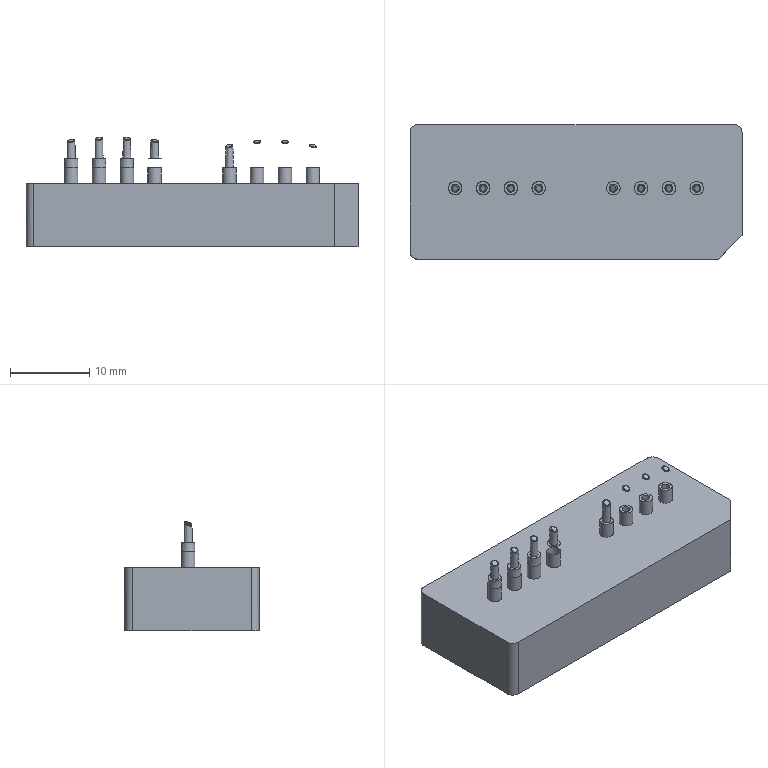NC program | PowerMill | posted by the shop | part box 42 x 17 x 13.856 mm
Lines 1 to 1570 of 273708:
%
G40 G49 G17 G80
( TOOL ID   D10C_1_1 )
( TOOL DIA. 10. TIP RAD 0 LENGTH 69.32 )
( Z = -.055 )
T1 M6
T15
G91 G28 Z0
G0 G90 G54
M08
S8000 M3
G0 X0 Y0 M8
G43 Z10.2 H1
X28.8 Y11.3
Z1.145
G1 Z-.055 F6000
X23.8 F10000
X-23.8
Y5.65
X23.8
Y0
X-23.8
Y-5.65
X23.8
Y-11.3
X-23.8
X-28.8
G0 Z10.2
X.006 Y0
Z9.895
X2.663 Y16.575
Z.711
G1 Z-.489 F6000
Y16.048 F10000
G3 X7.411 Y11.3 I4.747 J0
G1 X22.928
G2 X23.928 Y10.3 I0 J-1.
G1 Y-10.3
G2 X22.928 Y-11.3 I-1. J0
G1 X-22.916
G2 X-23.916 Y-10.3 I0 J1.
G1 Y10.3
G2 X-22.916 Y11.3 I1. J0
G1 X7.411
X7.934 Y6.084
X8.127 Y6.103
X8.9 Y6.063
X9.564 Y5.926
X9.623 Y5.918
X9.683 Y5.916
X9.856 Y5.864
X9.999 Y5.843
X10.142 Y5.863
X10.349 Y5.924
X10.382 Y5.921
X10.447
X10.512 Y5.928
X11.221 Y6.058
X11.994 Y6.099
X12.768 Y6.005
X13.541 Y5.771
X14.314 Y5.45
X15.088 Y4.943
X15.813 Y4.254
X16.367 Y3.48
X16.635 Y2.957
X16.732 Y2.707
X16.968 Y1.934
X17.072 Y1.16
X17.065 Y.387
X16.944 Y-.387
X16.635 Y-1.288
X16.296 Y-1.934
X15.721 Y-2.707
X15.088 Y-3.301
X14.849 Y-3.48
X14.314 Y-3.809
X13.541 Y-4.146
X13.228 Y-4.254
X12.768 Y-4.353
X11.994 Y-4.466
X11.221
X10.447 Y-4.344
X10.126 Y-4.264
X10.02 Y-4.25
X9.914 Y-4.258
X9.875 Y-4.261
X9.836 Y-4.267
X8.9 Y-4.457
X8.127 Y-4.472
X7.354 Y-4.382
X6.779 Y-4.254
X5.807 Y-3.87
X5.033 Y-3.398
X4.285 Y-2.707
X3.707 Y-1.934
X3.486 Y-1.537
X3.315 Y-1.16
X3.067 Y-.387
X2.933 Y.387
X2.922 Y1.16
X2.926 Y1.186
X.862 Y1.16
X.872 Y.387
X.768 Y-.387
X.547 Y-1.16
X.393 Y-1.526
X.186 Y-1.934
X-.342 Y-2.707
X-1.132 Y-3.48
X-1.928 Y-4.003
X-2.472 Y-4.254
X-3.474 Y-4.653
X-4.248 Y-4.836
X-5.021 Y-4.902
X-5.877 Y-4.83
X-5.984 Y-4.833
X-6.088 Y-4.858
X-6.56 Y-5.027
X-7.342 Y-5.207
X-8.115 Y-5.275
X-8.888 Y-5.238
X-9.662 Y-5.099
X-9.864 Y-5.042
X-9.999 Y-5.022
X-10.134 Y-5.04
X-10.435 Y-5.124
X-11.209 Y-5.249
X-11.982 Y-5.272
X-12.756 Y-5.191
X-13.441 Y-5.027
X-13.883 Y-4.868
X-13.995 Y-4.842
X-14.111
X-15.076 Y-4.901
X-15.849 Y-4.82
X-16.623 Y-4.622
X-17.533 Y-4.254
X-18.17 Y-3.948
X-18.863 Y-3.48
X-19.659 Y-2.707
X-20.188 Y-1.934
X-20.49 Y-1.307
X-20.768 Y-.387
X-20.868 Y.387
X-20.853 Y1.16
X-20.738 Y1.934
X-20.49 Y2.717
X-20.114 Y3.48
X-19.562 Y4.254
X-18.943 Y4.876
X-18.17 Y5.432
X-17.433 Y5.801
X-16.623 Y6.066
X-15.849 Y6.202
X-15.076 Y6.228
X-14.302 Y6.154
X-13.652 Y5.994
X-13.534 Y5.98
X-13.415 Y5.994
X-12.756 Y6.155
X-11.982 Y6.236
X-11.209 Y6.214
X-10.435 Y6.09
X-10.137 Y6.007
X-10.001 Y5.989
X-9.865 Y6.008
X-9.662 Y6.066
X-8.888 Y6.206
X-8.115 Y6.24
X-7.342 Y6.17
X-6.581 Y5.991
X-6.463 Y5.978
X-6.345 Y5.992
X-5.795 Y6.129
X-5.021 Y6.226
X-4.248 Y6.21
X-3.474 Y6.086
X-2.701 Y5.852
X-1.928 Y5.486
X-1.241 Y5.027
X-.445 Y4.254
X.111 Y3.48
X.491 Y2.707
X.736 Y1.934
X.862 Y1.16
X2.926 Y1.186
X3.039 Y1.934
X3.267 Y2.707
X3.636 Y3.48
X4.185 Y4.254
X5.033 Y5.038
X5.807 Y5.506
X6.477 Y5.801
X7.354 Y6.025
X7.934 Y6.084
X7.411 Y11.3
G0 Z3.326
G1 X2.663 Y16.575
G0 Z.326
G1 Z-.874 F6000
Y16.048 F10000
G3 X7.411 Y11.3 I4.747 J0
G1 X7.596
X8.03 Y6.214
X8.127 Y6.223
X8.9 Y6.185
X9.674 Y6.046
X9.866 Y5.992
X10. Y5.973
X10.134 Y5.991
X10.447 Y6.076
X11.221 Y6.192
X11.994 Y6.22
X12.768 Y6.139
X13.541 Y5.946
X13.936 Y5.801
X14.314 Y5.628
X15.088 Y5.168
X15.277 Y5.027
X15.861 Y4.506
X16.093 Y4.254
X16.635 Y3.527
X17.06 Y2.707
X17.323 Y1.934
X17.469 Y1.16
X17.507 Y.387
X17.44 Y-.387
X17.267 Y-1.16
X16.968 Y-1.934
X16.526 Y-2.707
X15.896 Y-3.48
X15.088 Y-4.17
X14.314 Y-4.631
X13.541 Y-4.938
X13.237 Y-5.027
X12.768 Y-5.132
X11.994 Y-5.222
X11.221 Y-5.206
X10.447 Y-5.079
X10.128 Y-4.999
X10.001 Y-4.984
X9.874 Y-5.002
X9.674 Y-5.057
X8.9 Y-5.192
X8.127 Y-5.225
X7.354 Y-5.155
X6.754 Y-5.027
X5.807 Y-4.682
X5.033 Y-4.256
X4.101 Y-3.48
X3.486 Y-2.73
X3.029 Y-1.934
X2.734 Y-1.16
X2.556 Y-.387
X2.491 Y.387
X2.5 Y.559
X1.043 Y.483
X1.048 Y.387
X.982 Y-.387
X.812 Y-1.16
X.517 Y-1.934
X.393 Y-2.194
X.091 Y-2.707
X-.381 Y-3.324
X-1.154 Y-4.059
X-1.419 Y-4.254
X-1.928 Y-4.565
X-2.701 Y-4.924
X-2.994 Y-5.027
X-3.474 Y-5.156
X-4.248 Y-5.268
X-5.021 Y-5.282
X-5.795 Y-5.195
X-6.364 Y-5.05
X-6.483 Y-5.035
X-6.601 Y-5.048
X-7.342 Y-5.221
X-8.115 Y-5.294
X-8.888 Y-5.256
X-9.662 Y-5.112
X-9.87 Y-5.055
X-10.001 Y-5.037
X-10.133 Y-5.054
X-10.435 Y-5.136
X-11.209 Y-5.267
X-11.982 Y-5.291
X-12.756 Y-5.205
X-13.399 Y-5.049
X-13.517 Y-5.035
X-13.636 Y-5.049
X-14.302 Y-5.212
X-15.076 Y-5.29
X-15.849 Y-5.266
X-16.623 Y-5.133
X-17.008 Y-5.027
X-17.396 Y-4.889
X-18.17 Y-4.514
X-18.584 Y-4.254
X-18.943 Y-3.979
X-19.479 Y-3.48
X-19.716 Y-3.212
X-20.091 Y-2.707
X-20.49 Y-1.993
X-20.808 Y-1.16
X-20.977 Y-.387
X-21.044 Y.387
X-21.009 Y1.16
X-20.861 Y1.934
X-20.599 Y2.707
X-20.203 Y3.48
X-19.716 Y4.166
X-18.943 Y4.928
X-18.17 Y5.473
X-17.505 Y5.801
X-16.623 Y6.084
X-15.849 Y6.221
X-15.076 Y6.245
X-14.302 Y6.163
X-13.639 Y6.004
X-13.521 Y5.99
X-13.404 Y6.004
X-12.756 Y6.163
X-11.982 Y6.238
X-11.209 Y6.218
X-10.435 Y6.097
X-10.137 Y6.014
X-10.001 Y5.995
X-9.865 Y6.015
X-9.662 Y6.073
X-8.888 Y6.21
X-8.115 Y6.241
X-7.342 Y6.179
X-6.596 Y6.002
X-6.478 Y5.989
X-6.36 Y6.004
X-5.795 Y6.145
X-5.021 Y6.241
X-4.248 Y6.23
X-3.474 Y6.106
X-2.701 Y5.881
X-1.928 Y5.527
X-1.154 Y5.011
X-.381 Y4.279
X.204 Y3.48
X.393 Y3.148
X.6 Y2.707
X.862 Y1.934
X1.008 Y1.16
X1.043 Y.483
X2.5 Y.559
X2.53 Y1.16
X2.677 Y1.934
X2.939 Y2.707
X3.336 Y3.48
X3.486 Y3.712
X3.905 Y4.254
X4.26 Y4.631
X4.722 Y5.027
X5.033 Y5.252
X5.807 Y5.687
X6.58 Y5.983
X7.354 Y6.157
X8.03 Y6.214
X7.596 Y11.3
X22.928
G2 X23.928 Y10.3 I0 J-1.
G1 Y-10.3
G2 X22.928 Y-11.3 I-1. J0
G1 X-22.916
G2 X-23.916 Y-10.3 I0 J1.
G1 Y10.3
G2 X-22.916 Y11.3 I1. J0
G1 X7.411
G0 Z2.942
G1 X2.663 Y16.575
G0 Z-.058
G1 Z-1.258 F6000
Y16.048 F10000
G3 X7.411 Y11.3 I4.747 J0
G1 X22.928
G2 X23.928 Y10.3 I0 J-1.
G1 Y-10.3
G2 X22.928 Y-11.3 I-1. J0
G1 X-22.916
G2 X-23.916 Y-10.3 I0 J1.
G1 Y.51
X-21.048 Y.387
X-21.015 Y1.16
X-20.868 Y1.934
X-20.602 Y2.707
X-20.213 Y3.48
X-19.716 Y4.176
X-18.943 Y4.935
X-18.17 Y5.481
X-17.523 Y5.801
X-16.623 Y6.089
X-15.849 Y6.228
X-15.076 Y6.253
X-14.302 Y6.164
X-13.64 Y6.009
X-13.523 Y5.996
X-13.406 Y6.01
X-12.756 Y6.17
X-11.982 Y6.243
X-11.209 Y6.225
X-10.435 Y6.104
X-10.137 Y6.021
X-10.001 Y6.002
X-9.865 Y6.022
X-9.662 Y6.08
X-8.888 Y6.216
X-8.115 Y6.244
X-7.342 Y6.185
X-6.595 Y6.009
X-6.478 Y5.995
X-6.36 Y6.01
X-5.795 Y6.149
X-5.021 Y6.248
X-4.248 Y6.237
X-3.474 Y6.114
X-2.701 Y5.888
X-1.928 Y5.536
X-1.166 Y5.027
X-.35 Y4.254
G3 X.386 Y4.254 I.368 J.339
G1 X1.166 Y5.002
X1.94 Y5.518
X2.527 Y5.801
X3.486 Y6.096
X4.26 Y6.212
X5.033 Y6.224
X5.807 Y6.131
X6.366 Y5.99
X6.476 Y5.975
X6.586 Y5.985
X6.611 Y5.99
X7.354 Y6.168
X8.127 Y6.231
X8.9 Y6.19
X9.674 Y6.054
X9.866 Y5.999
X10. Y5.98
X10.134 Y5.998
X10.447 Y6.083
X11.221 Y6.199
X11.994 Y6.228
X12.768 Y6.147
X13.395 Y5.99
X13.514 Y5.975
X13.633 Y5.989
X14.314 Y6.152
X15.088 Y6.227
X15.861 Y6.2
X16.635 Y6.066
X17.408 Y5.824
X18.182 Y5.449
X18.806 Y5.027
X19.614 Y4.254
X20.171 Y3.48
X20.502 Y2.847
X20.813 Y1.934
X20.946 Y1.16
X20.972 Y.387
X20.886 Y-.387
X20.681 Y-1.16
X20.502 Y-1.62
X20.348 Y-1.934
X19.859 Y-2.707
X19.728 Y-2.873
X19.149 Y-3.48
X18.955 Y-3.643
X18.182 Y-4.161
X17.408 Y-4.545
X16.635 Y-4.855
X15.915 Y-5.027
X15.088 Y-5.096
X14.314 Y-5.045
X13.855 Y-4.959
X13.719 Y-4.952
X13.587 Y-4.982
X13.541 Y-4.999
X12.768 Y-5.192
X11.994 Y-5.275
X11.221 Y-5.254
X10.447 Y-5.124
X10.133 Y-5.041
X10. Y-5.024
X9.868 Y-5.043
X9.674 Y-5.098
X8.9 Y-5.24
X8.127 Y-5.28
X7.354 Y-5.211
X6.562 Y-5.027
X6.411 Y-4.975
X6.284 Y-4.95
X6.154 Y-4.958
X5.795 Y-5.027
X5.033 Y-5.092
X4.26 Y-5.049
X3.486 Y-4.888
X2.713 Y-4.598
X1.94 Y-4.221
X1.166 Y-3.732
X.86 Y-3.48
X.489 Y-3.11
G3 X-.214 Y-3.105 I-.353 J-.354
G1 X-.381 Y-3.324
X-.415 Y-3.357
X-.512 Y-3.48
X-1.154 Y-4.06
X-1.172 Y-4.072
X-1.419 Y-4.254
X-1.7 Y-4.426
X-1.928 Y-4.578
X-2.701 Y-4.936
X-2.893 Y-4.991
X-2.994 Y-5.027
X-3.313 Y-5.113
X-3.474 Y-5.159
X-4.248 Y-5.281
X-5.021 Y-5.294
X-5.795 Y-5.195
X-6.354 Y-5.057
X-6.469 Y-5.043
X-6.584 Y-5.055
X-7.342 Y-5.227
X-8.115 Y-5.301
X-8.888 Y-5.263
X-9.662 Y-5.117
X-9.872 Y-5.06
X-10.001 Y-5.042
X-10.13 Y-5.058
X-10.435 Y-5.138
X-11.209 Y-5.274
X-11.982 Y-5.298
X-12.756 Y-5.209
X-13.404 Y-5.052
X-13.522 Y-5.038
X-13.639 Y-5.052
X-14.302 Y-5.213
X-15.076 Y-5.298
X-15.849 Y-5.273
X-16.623 Y-5.14
X-16.818 Y-5.079
X-17.008 Y-5.027
X-17.158 Y-4.973
X-17.396 Y-4.9
X-18.17 Y-4.521
X-18.591 Y-4.254
X-18.943 Y-3.987
X-19.488 Y-3.48
X-19.716 Y-3.222
X-20.094 Y-2.707
X-20.49 Y-2.002
X-20.819 Y-1.16
X-20.987 Y-.387
X-21.048 Y.387
X-23.916 Y.51
Y10.3
G2 X-22.916 Y11.3 I1. J0
G1 X7.411
G0 Z2.558
G1 X2.663 Y16.575
G0 Z-.442
G1 Z-1.642 F6000
Y16.048 F10000
G3 X7.411 Y11.3 I4.747 J0
G1 X22.928
G2 X23.928 Y10.3 I0 J-1.
G1 Y-10.3
G2 X22.928 Y-11.3 I-1. J0
G1 X-22.916
G2 X-23.916 Y-10.3 I0 J1.
G1 Y.503
X-21.053 Y.387
X-21.021 Y1.16
X-20.875 Y1.934
X-20.605 Y2.707
X-20.22 Y3.48
X-19.716 Y4.187
X-18.943 Y4.941
X-18.17 Y5.488
X-17.541 Y5.801
X-16.623 Y6.095
X-15.849 Y6.234
X-15.076 Y6.26
X-14.302 Y6.171
X-13.639 Y6.016
X-13.523 Y6.003
X-13.406 Y6.017
X-12.756 Y6.177
X-11.982 Y6.25
X-11.209 Y6.232
X-10.435 Y6.111
X-10.137 Y6.028
X-10.001 Y6.009
X-9.865 Y6.029
X-9.662 Y6.087
X-8.888 Y6.223
X-8.115 Y6.251
X-7.342 Y6.192
X-6.594 Y6.015
X-6.478 Y6.002
X-6.361 Y6.016
X-5.795 Y6.154
X-5.021 Y6.255
X-4.248 Y6.244
X-3.474 Y6.12
X-2.701 Y5.895
X-1.928 Y5.543
X-1.157 Y5.027
X-.341 Y4.254
G3 X.393 Y4.278 I.356 J.352
G1 X1.166 Y5.015
X1.94 Y5.518
X1.979 Y5.537
X2.528 Y5.801
X2.574 Y5.815
X2.713 Y5.88
X3.486 Y6.109
X4.26 Y6.22
X5.033 Y6.231
X5.807 Y6.14
X6.366 Y5.998
X6.485 Y5.982
X6.605 Y5.996
X7.354 Y6.174
X8.127 Y6.238
X8.9 Y6.194
X9.674 Y6.061
X9.866 Y6.006
X10. Y5.987
X10.134 Y6.005
X10.447 Y6.09
X11.221 Y6.205
X11.994 Y6.235
X12.768 Y6.154
X13.393 Y5.997
X13.513 Y5.982
X13.633 Y5.996
X14.314 Y6.162
X15.088 Y6.233
X15.861 Y6.211
X16.635 Y6.08
X17.408 Y5.832
X18.182 Y5.452
X18.386 Y5.311
X18.805 Y5.027
X18.832 Y5.002
X18.955 Y4.917
X19.626 Y4.254
X20.194 Y3.48
X20.593 Y2.707
X20.853 Y1.934
X20.998 Y1.16
X21.04 Y.387
X20.974 Y-.387
X20.8 Y-1.16
X20.502 Y-1.955
X20.082 Y-2.707
X19.728 Y-3.182
X19.462 Y-3.48
X18.955 Y-3.957
X18.571 Y-4.254
X18.182 Y-4.501
X17.408 Y-4.877
X16.988 Y-5.027
X16.635 Y-5.122
X15.861 Y-5.256
X15.088 Y-5.282
X14.314 Y-5.204
X13.631 Y-5.04
X13.511 Y-5.026
X13.391 Y-5.041
X12.768 Y-5.199
X11.994 Y-5.283
X11.221 Y-5.261
X10.447 Y-5.131
X10.133 Y-5.047
X10. Y-5.03
X9.868 Y-5.049
X9.674 Y-5.103
X8.9 Y-5.247
X8.127 Y-5.287
X7.354 Y-5.219
X6.609 Y-5.04
X6.489 Y-5.026
X6.37 Y-5.041
X5.807 Y-5.183
X5.033 Y-5.279
X4.26 Y-5.267
X3.486 Y-5.149
X3.01 Y-5.027
X2.713 Y-4.924
X1.94 Y-4.568
X1.435 Y-4.254
X1.166 Y-4.057
X.534 Y-3.48
X.408 Y-3.327
G3 X-.373 Y-3.336 I-.386 J-.317
G1 X-.381 Y-3.346
X-.478 Y-3.438
X-.512 Y-3.48
X-.908 Y-3.838
X-1.154 Y-4.068
X-1.284 Y-4.155
X-1.419 Y-4.254
X-1.57 Y-4.346
X-1.928 Y-4.586
X-2.701 Y-4.943
X-2.985 Y-5.024
X-2.994 Y-5.027
X-3.029 Y-5.037
X-3.474 Y-5.163
X-4.248 Y-5.288
X-5.021 Y-5.301
X-5.795 Y-5.2
X-6.368 Y-5.06
X-6.484 Y-5.046
X-6.601 Y-5.059
X-7.342 Y-5.234
X-8.115 Y-5.308
X-8.888 Y-5.269
X-9.662 Y-5.122
X-9.872 Y-5.065
X-10. Y-5.048
X-10.128 Y-5.064
X-10.435 Y-5.143
X-11.209 Y-5.281
X-11.982 Y-5.305
X-12.756 Y-5.216
X-13.402 Y-5.059
X-13.519 Y-5.045
X-13.637 Y-5.059
X-14.302 Y-5.219
X-15.076 Y-5.305
X-15.849 Y-5.28
X-16.623 Y-5.144
X-16.967 Y-5.038
X-17.008 Y-5.027
X-17.034 Y-5.018
X-17.396 Y-4.907
X-18.17 Y-4.529
X-18.598 Y-4.254
X-18.943 Y-3.994
X-19.497 Y-3.48
X-19.716 Y-3.233
X-20.101 Y-2.707
X-20.49 Y-2.015
X-20.826 Y-1.16
X-20.994 Y-.387
X-21.053 Y.387
X-23.916 Y.503
Y10.3
G2 X-22.916 Y11.3 I1. J0
G1 X7.411
G0 Z2.173
G1 X2.663 Y16.575
G0 Z-.827
G1 Z-2.027 F6000
Y16.048 F10000
G3 X7.411 Y11.3 I4.747 J0
G1 X22.928
G2 X23.928 Y10.3 I0 J-1.
G1 Y-10.3
G2 X22.928 Y-11.3 I-1. J0
G1 X-22.916
G2 X-23.916 Y-10.3 I0 J1.
G1 Y.499
X-21.059 Y.387
X-21.028 Y1.16
X-20.882 Y1.934
X-20.612 Y2.707
X-20.228 Y3.48
X-19.716 Y4.197
X-18.943 Y4.949
X-18.17 Y5.496
X-17.558 Y5.801
X-16.623 Y6.101
X-15.849 Y6.241
X-15.076 Y6.266
X-14.302 Y6.178
X-13.639 Y6.023
X-13.523 Y6.009
X-13.406 Y6.024
X-12.756 Y6.183
X-11.982 Y6.256
X-11.209 Y6.238
X-10.435 Y6.118
X-10.137 Y6.035
X-10.001 Y6.016
X-9.865 Y6.036
X-9.662 Y6.094
X-8.888 Y6.229
X-8.115 Y6.258
X-7.342 Y6.199
X-6.594 Y6.022
X-6.478 Y6.009
X-6.362 Y6.023
X-5.795 Y6.159
X-5.021 Y6.262
X-4.248 Y6.25
X-3.474 Y6.126
X-2.701 Y5.902
X-1.928 Y5.551
X-1.154 Y5.032
X-.332 Y4.254
G3 X.393 Y4.287 I.346 J.36
G1 X1.166 Y5.023
X1.94 Y5.525
X2.463 Y5.77
X2.528 Y5.801
X2.533 Y5.802
X2.713 Y5.886
X3.486 Y6.116
X4.26 Y6.227
X5.033 Y6.237
X5.807 Y6.146
X6.367 Y6.004
X6.487 Y5.989
X6.607 Y6.002
X7.354 Y6.181
X8.127 Y6.244
X8.9 Y6.201
X9.674 Y6.068
X9.867 Y6.013
X10. Y5.994
X10.134 Y6.012
X10.447 Y6.097
X11.221 Y6.212
X11.994 Y6.242
X12.768 Y6.161
X13.392 Y6.004
X13.512 Y5.989
X13.632 Y6.003
X14.314 Y6.168
X15.088 Y6.239
X15.861 Y6.218
X16.635 Y6.087
X17.408 Y5.839
X18.182 Y5.46
X18.828 Y5.027
X18.914 Y4.945
X18.955 Y4.917
X19.344 Y4.532
X19.634 Y4.254
X20.202 Y3.48
X20.6 Y2.707
X20.859 Y1.934
X21.001 Y1.16
X21.048 Y.387
X20.982 Y-.387
X20.806 Y-1.16
X20.519 Y-1.934
X20.09 Y-2.707
X19.728 Y-3.191
X19.466 Y-3.48
X18.955 Y-3.966
X18.582 Y-4.254
X18.182 Y-4.51
X17.408 Y-4.884
X17.012 Y-5.027
X16.635 Y-5.132
X15.861 Y-5.263
X15.088 Y-5.291
X14.314 Y-5.207
X13.632 Y-5.045
X13.513 Y-5.032
X13.394 Y-5.047
X12.768 Y-5.206
X11.994 Y-5.29
X11.221 Y-5.267
X10.447 Y-5.137
X10.131 Y-5.053
X10. Y-5.036
X9.869 Y-5.054
X9.674 Y-5.108
X8.9 Y-5.254
X8.127 Y-5.294
X7.354 Y-5.226
X6.586 Y-5.048
X6.47 Y-5.035
X6.354 Y-5.05
X5.807 Y-5.183
X5.033 Y-5.286
X4.26 Y-5.274
X3.486 Y-5.16
X3.22 Y-5.081
X3.01 Y-5.027
X2.853 Y-4.973
X2.713 Y-4.932
X1.94 Y-4.578
X1.419 Y-4.254
X1.166 Y-4.064
X.94 Y-3.85
X.534 Y-3.48
X.485 Y-3.42
X.393 Y-3.333
G3 X-.378 Y-3.353 I-.377 J-.328
G1 X-.381 Y-3.357
X-.506 Y-3.473
X-.512 Y-3.48
X-.59 Y-3.551
X-1.154 Y-4.075
X-1.398 Y-4.238
X-1.419 Y-4.254
X-1.442 Y-4.268
X-1.928 Y-4.593
X-2.701 Y-4.951
X-3.474 Y-5.17
X-4.248 Y-5.294
X-5.021 Y-5.307
X-5.795 Y-5.207
X-6.369 Y-5.066
X-6.486 Y-5.051
X-6.603 Y-5.065
X-7.342 Y-5.24
X-8.115 Y-5.314
X-8.888 Y-5.276
X-9.662 Y-5.127
X-9.873 Y-5.071
X-10. Y-5.054
X-10.127 Y-5.069
X-10.435 Y-5.149
X-11.209 Y-5.287
X-11.982 Y-5.311
X-12.756 Y-5.223
X-13.398 Y-5.065
X-13.516 Y-5.051
X-13.634 Y-5.065
X-14.302 Y-5.226
X-15.076 Y-5.312
X-15.849 Y-5.286
X-16.623 Y-5.15
X-17.396 Y-4.914
X-18.17 Y-4.536
X-18.605 Y-4.254
X-18.943 Y-4.002
X-19.507 Y-3.48
X-19.716 Y-3.243
X-20.109 Y-2.707
X-20.49 Y-2.029
X-20.833 Y-1.16
X-21.001 Y-.387
X-21.059 Y.387
X-23.916 Y.499
Y10.3
G2 X-22.916 Y11.3 I1. J0
G1 X7.411
G0 Z1.789
G1 X2.663 Y16.575
G0 Z-1.211
G1 Z-2.411 F6000
Y16.048 F10000
G3 X7.411 Y11.3 I4.747 J0
G1 X22.928
G2 X23.928 Y10.3 I0 J-1.
G1 Y-10.3
G2 X22.928 Y-11.3 I-1. J0
G1 X-22.916
G2 X-23.916 Y-10.3 I0 J1.
G1 Y.498
X-21.065 Y.387
X-21.035 Y1.16
X-20.889 Y1.934
X-20.618 Y2.707
X-20.236 Y3.48
X-19.716 Y4.207
X-18.943 Y4.957
X-18.17 Y5.504
X-17.575 Y5.801
X-16.623 Y6.107
X-15.849 Y6.248
X-15.076 Y6.273
X-14.302 Y6.184
X-13.639 Y6.029
X-13.523 Y6.016
X-13.406 Y6.031
X-12.756 Y6.19
X-11.982 Y6.263
X-11.209 Y6.245
X-10.435 Y6.124
X-10.137 Y6.042
X-10.001 Y6.023
X-9.865 Y6.043
X-9.662 Y6.101
X-8.888 Y6.236
X-8.115 Y6.264
X-7.342 Y6.206
X-6.594 Y6.029
X-6.478 Y6.016
X-6.362 Y6.029
X-5.795 Y6.166
X-5.021 Y6.268
X-4.248 Y6.257
X-3.474 Y6.132
X-2.701 Y5.909
X-2.424 Y5.801
X-1.928 Y5.559
X-1.154 Y5.039
X-.381 Y4.319
X-.376 Y4.313
G3 X.393 Y4.296 I.392 J.311
G1 X1.161 Y5.027
X1.94 Y5.533
X2.713 Y5.893
X3.486 Y6.122
X4.26 Y6.234
X5.033 Y6.242
X5.807 Y6.153
X6.369 Y6.01
X6.489 Y5.995
X6.609 Y6.009
X7.354 Y6.188
X8.127 Y6.251
X8.9 Y6.207
X9.674 Y6.075
X9.867 Y6.02
X10. Y6.001
X10.134 Y6.019
X10.447 Y6.103
X11.221 Y6.218
X11.994 Y6.249
X12.768 Y6.168
X13.391 Y6.011
X13.511 Y5.995
X13.63 Y6.009
X14.314 Y6.174
X15.088 Y6.244
X15.861 Y6.225
X16.635 Y6.094
X17.408 Y5.844
X18.182 Y5.468
X18.839 Y5.027
X18.952 Y4.919
X18.955 Y4.917
X18.985 Y4.887
X19.642 Y4.254
X20.21 Y3.48
X20.608 Y2.707
X20.865 Y1.934
X21.008 Y1.16
X21.054 Y.387
X20.989 Y-.387
X20.811 Y-1.16
X20.526 Y-1.934
X20.098 Y-2.707
X19.728 Y-3.2
X19.474 Y-3.48
X18.955 Y-3.975
X18.594 Y-4.254
X18.182 Y-4.517
X17.408 Y-4.892
X17.034 Y-5.027
X16.635 Y-5.139
X15.861 Y-5.27
X15.088 Y-5.298
X14.314 Y-5.213
X13.633 Y-5.052
X13.514 Y-5.038
X13.395 Y-5.054
X12.768 Y-5.213
X11.994 Y-5.296
X11.221 Y-5.274
X10.447 Y-5.142
X10.13 Y-5.058
X10. Y-5.042
X9.87 Y-5.06
X9.674 Y-5.114
X8.9 Y-5.26
X8.127 Y-5.3
X7.354 Y-5.233
X6.645 Y-5.062
X6.586 Y-5.048
X6.582 Y-5.047
X6.578
X6.473 Y-5.038
X6.368 Y-5.052
X5.807 Y-5.19
X5.033 Y-5.292
X4.26 Y-5.281
X3.486 Y-5.166
X3.037 Y-5.034
X3.01 Y-5.027
X2.99 Y-5.02
X2.713 Y-4.939
X1.94 Y-4.586
X1.407 Y-4.254
X1.166 Y-4.073
X.685 Y-3.618
X.534 Y-3.48
X.516 Y-3.458
X.393 Y-3.342
G3 X-.377 Y-3.362 I-.376 J-.329
G1 X-.381 Y-3.367
X-1.154 Y-4.082
X-1.928 Y-4.601
X-2.701 Y-4.958
X-3.474 Y-5.176
X-4.248 Y-5.301
X-5.021 Y-5.314
X-5.795 Y-5.213
X-6.37 Y-5.072
X-6.487 Y-5.057
X-6.605 Y-5.071
X-7.342 Y-5.247
X-8.115 Y-5.321
X-8.888 Y-5.283
X-9.662 Y-5.132
X-9.873 Y-5.076
X-10. Y-5.059
X-10.127 Y-5.075
X-10.435 Y-5.155
X-11.209 Y-5.294
X-11.982 Y-5.318
X-12.756 Y-5.229
X-13.395 Y-5.072
X-13.513 Y-5.057
X-13.632 Y-5.071
X-14.302 Y-5.232
X-15.076 Y-5.319
X-15.849 Y-5.292
X-16.623 Y-5.157
X-17.396 Y-4.921
X-18.17 Y-4.544
X-18.351 Y-4.419
X-18.605 Y-4.254
X-18.808 Y-4.103
X-18.943 Y-4.009
X-19.516 Y-3.48
X-19.716 Y-3.254
X-20.117 Y-2.707
X-20.49 Y-2.044
X-20.84 Y-1.16
X-21.007 Y-.387
X-21.065 Y.387
X-23.916 Y.498
Y10.3
G2 X-22.916 Y11.3 I1. J0
G1 X7.411
G0 Z1.405
G1 X2.663 Y16.575
G0 Z-1.595
G1 Z-2.795 F6000
Y16.048 F10000
G3 X7.411 Y11.3 I4.747 J0
G1 X22.928
G2 X23.928 Y10.3 I0 J-1.
G1 Y-10.3
G2 X22.928 Y-11.3 I-1. J0
G1 X-22.916
G2 X-23.916 Y-10.3 I0 J1.
G1 Y-.074
X-21.361 Y.097
X-21.381 Y.387
X-21.347 Y1.16
X-21.263 Y1.722
X-20.963 Y2.707
X-20.602 Y3.48
X-20.08 Y4.254
X-19.716 Y4.68
X-19.354 Y5.027
X-18.943 Y5.371
X-18.281 Y5.801
X-17.396 Y6.204
X-16.623 Y6.429
X-15.849 Y6.56
X-15.076 Y6.586
X-14.302 Y6.514
X-13.632 Y6.36
X-13.521 Y6.347
X-13.41 Y6.36
X-12.756 Y6.508
X-12.201 Y6.574
X-11.291
X-10.435 Y6.448
X-10.136 Y6.369
X-10.004 Y6.353
X-9.872 Y6.372
X-9.849 Y6.378
X-8.67 Y6.574
X-7.769
X-7.342 Y6.517
X-6.668 Y6.369
X-6.616 Y6.36
X-6.562 Y6.357
X-6.463 Y6.35
X-6.365 Y6.362
X-5.795 Y6.492
X-5.165 Y6.574
X-4.248 Y6.575
X-3.474 Y6.455
X-2.701 Y6.237
X-1.928 Y5.915
X-1.154 Y5.438
X-.641 Y5.027
X-.381 Y4.781
X-.152 Y4.514
G3 X.573 Y4.477 I.38 J.325
G1 X1.15 Y5.027
X1.94 Y5.54
X2.713 Y5.899
X3.486 Y6.129
X4.26 Y6.241
X5.033 Y6.247
X5.807 Y6.16
X6.369 Y6.017
X6.489 Y6.002
X6.608 Y6.016
X7.354 Y6.195
X8.127 Y6.258
X8.9 Y6.214
X9.674 Y6.082
X9.867 Y6.027
X10. Y6.008
X10.133 Y6.025
X10.447 Y6.11
X11.221 Y6.225
X11.994 Y6.255
X12.768 Y6.174
X13.39 Y6.017
X13.51 Y6.002
X13.63 Y6.016
X14.314 Y6.18
X15.088 Y6.249
X15.861 Y6.232
X16.635 Y6.101
X17.408 Y5.85
X18.182 Y5.475
X18.85 Y5.027
X19.65 Y4.254
X20.218 Y3.48
X20.502 Y2.96
X20.615 Y2.707
X20.871 Y1.934
X21.015 Y1.16
X21.061 Y.387
X20.995 Y-.387
X20.816 Y-1.16
X20.533 Y-1.934
X20.106 Y-2.707
X19.728 Y-3.209
X19.481 Y-3.48
X18.955 Y-3.984
X18.605 Y-4.254
X18.182 Y-4.525
X17.408 Y-4.899
X17.056 Y-5.027
X16.635 Y-5.146
X15.861 Y-5.277
X15.088 Y-5.305
X14.314 Y-5.22
X13.636 Y-5.059
X13.516 Y-5.045
X13.397 Y-5.06
X12.768 Y-5.22
X11.994 Y-5.303
X11.221 Y-5.281
X10.447 Y-5.147
X10.13 Y-5.064
X10. Y-5.048
X9.871 Y-5.065
X9.674 Y-5.119
X8.9 Y-5.267
X8.127 Y-5.307
X7.354 Y-5.24
X6.602 Y-5.058
X6.484 Y-5.045
X6.366 Y-5.059
X5.807 Y-5.196
X5.033 Y-5.299
X4.26 Y-5.288
X3.486 Y-5.173
X2.713 Y-4.946
X1.94 Y-4.593
X1.396 Y-4.254
X1.166 Y-4.081
X.558 Y-3.52
G3 X-.161 Y-3.564 I-.339 J-.368
G1 X-.381 Y-3.821
X-.855 Y-4.254
X-1.154 Y-4.479
X-1.928 Y-4.962
X-2.701 Y-5.288
X-3.474 Y-5.505
X-4.248 Y-5.619
X-5.021 Y-5.622
X-5.795 Y-5.538
X-6.374 Y-5.405
X-6.485 Y-5.392
X-6.595 Y-5.404
X-7.342 Y-5.57
X-8.115 Y-5.633
X-8.888 Y-5.596
X-9.662 Y-5.47
X-9.876 Y-5.413
X-10.001 Y-5.396
X-10.127 Y-5.412
X-10.435 Y-5.49
X-11.209 Y-5.612
X-11.982 Y-5.628
X-12.756 Y-5.55
X-13.141 Y-5.479
X-13.419 Y-5.406
X-13.541 Y-5.389
X-13.663 Y-5.403
X-14.302 Y-5.555
X-15.076 Y-5.629
X-15.849 Y-5.604
X-16.623 Y-5.481
X-17.396 Y-5.257
X-18.17 Y-4.908
X-18.943 Y-4.413
X-19.149 Y-4.254
X-19.716 Y-3.719
X-19.924 Y-3.48
X-20.49 Y-2.718
X-20.894 Y-1.934
X-21.167 Y-1.16
X-21.329 Y-.387
X-21.361 Y.097
X-23.916 Y-.074
Y10.3
G2 X-22.916 Y11.3 I1. J0
G1 X7.411
G0 Z1.02
G1 X2.663 Y16.575
G0 Z-1.98
G1 Z-3.18 F6000
Y16.048 F10000
G3 X7.411 Y11.3 I4.747 J0
G1 X22.928
G2 X23.928 Y10.3 I0 J-1.
G1 Y-10.3
G2 X22.928 Y-11.3 I-1. J0
G1 X-22.916
G2 X-23.916 Y-10.3 I0 J1.
G1 Y.519
X-21.412 Y.387
X-21.372 Y1.16
X-21.263 Y1.834
X-20.992 Y2.707
X-20.625 Y3.48
X-20.49 Y3.714
X-20.118 Y4.254
X-19.716 Y4.71
X-19.387 Y5.027
X-18.943 Y5.398
X-18.336 Y5.801
X-17.396 Y6.228
X-16.623 Y6.468
X-15.987 Y6.574
X-15.076 Y6.606
X-14.302 Y6.54
X-13.633 Y6.382
X-13.519 Y6.369
X-13.404 Y6.382
X-12.756 Y6.535
X-11.982 Y6.609
X-11.209 Y6.59
X-10.435 Y6.473
X-10.134 Y6.391
X-10.001 Y6.374
X-9.868 Y6.392
X-9.662 Y6.45
X-8.952 Y6.574
X-8.115 Y6.608
X-7.53 Y6.574
X-6.594 Y6.378
X-6.483 Y6.368
X-6.373 Y6.382
X-5.795 Y6.523
X-5.021 Y6.602
X-4.248 Y6.596
X-3.474 Y6.489
X-2.701 Y6.263
X-1.928 Y5.941
X-1.664 Y5.801
X-1.154 Y5.471
X-.381 Y4.809
X-.129 Y4.529
G3 X.588 Y4.501 I.372 J.334
G1 X1.139 Y5.027
X1.94 Y5.547
X2.713 Y5.905
X3.486 Y6.136
X4.26 Y6.247
X5.033 Y6.252
X5.807 Y6.166
X6.37 Y6.024
X6.49 Y6.009
X6.61 Y6.023
X7.354 Y6.201
X8.127 Y6.264
X8.9 Y6.221
X9.674 Y6.089
X9.867 Y6.034
X10. Y6.015
X10.133 Y6.032
X10.447 Y6.117
X11.221 Y6.231
X11.994 Y6.262
X12.768 Y6.181
X13.389 Y6.024
X13.509 Y6.009
X13.628 Y6.022
X14.314 Y6.187
X15.088 Y6.254
X15.861 Y6.238
X16.635 Y6.108
X17.408 Y5.856
X18.182 Y5.483
X18.861 Y5.027
X19.658 Y4.254
X20.225 Y3.48
X20.502 Y2.976
X20.622 Y2.707
X20.877 Y1.934
X21.021 Y1.16
X21.068 Y.387
X21.002 Y-.387
X20.82 Y-1.16
X20.541 Y-1.934
X20.114 Y-2.707
X19.728 Y-3.218
X19.489 Y-3.48
X18.955 Y-3.992
X18.617 Y-4.254
X18.182 Y-4.533
X17.408 Y-4.906
X17.077 Y-5.027
X16.635 Y-5.153
X15.861 Y-5.283
X15.088 Y-5.312
X14.314 Y-5.227
X13.638 Y-5.065
X13.519 Y-5.052
X13.4 Y-5.067
X12.768 Y-5.226
X11.994 Y-5.31
X11.221 Y-5.288
X10.447 Y-5.152
X10.129 Y-5.069
X10. Y-5.053
X9.872 Y-5.071
X9.674 Y-5.125
X8.9 Y-5.274
X8.127 Y-5.314
X7.354 Y-5.246
X6.601 Y-5.065
X6.483 Y-5.051
X6.364 Y-5.066
X5.807 Y-5.203
X5.033 Y-5.306
X4.26 Y-5.295
X3.486 Y-5.18
X2.713 Y-4.953
X1.94 Y-4.601
X1.384 Y-4.254
X1.166 Y-4.09
X.582 Y-3.549
G3 X-.129 Y-3.582 I-.34 J-.367
G1 X-.381 Y-3.862
X-.812 Y-4.254
X-1.154 Y-4.51
X-1.928 Y-4.983
X-2.701 Y-5.32
X-3.474 Y-5.525
X-4.248 Y-5.641
X-5.021 Y-5.654
X-5.795 Y-5.559
X-6.374 Y-5.427
X-6.482 Y-5.415
X-6.591 Y-5.426
X-7.342 Y-5.589
X-8.115 Y-5.661
X-8.888 Y-5.623
X-9.662 Y-5.489
X-9.877 Y-5.434
X-9.999 Y-5.418
X-10.12 Y-5.433
X-10.435 Y-5.511
X-11.209 Y-5.634
X-11.982 Y-5.658
X-12.756 Y-5.571
X-13.409 Y-5.426
X-13.517 Y-5.415
X-13.625 Y-5.426
X-14.302 Y-5.576
X-15.076 Y-5.659
X-15.849 Y-5.632
X-16.623 Y-5.507
X-17.396 Y-5.284
X-17.988 Y-5.027
X-18.943 Y-4.442
X-19.188 Y-4.254
X-19.716 Y-3.76
X-19.96 Y-3.48
X-20.49 Y-2.758
X-20.921 Y-1.934
X-21.181 Y-1.16
X-21.354 Y-.387
X-21.412 Y.387
X-23.916 Y.519
Y10.3
G2 X-22.916 Y11.3 I1. J0
G1 X7.411
G0 Z.636
G1 X2.663 Y16.575
G0 Z-2.364
G1 Z-3.564 F6000
Y16.048 F10000
G3 X7.411 Y11.3 I4.747 J0
G1 X22.928
G2 X23.928 Y10.3 I0 J-1.
G1 Y-10.3
G2 X22.928 Y-11.3 I-1. J0
G1 X-22.916
G2 X-23.916 Y-10.3 I0 J1.
G1 Y.534
X-21.42 Y.387
X-21.374 Y1.16
X-21.263 Y1.865
X-21. Y2.707
X-20.842 Y3.023
X-20.625 Y3.48
X-20.538 Y3.63
X-20.49 Y3.727
X-20.126 Y4.254
X-19.716 Y4.719
X-19.59 Y4.831
X-19.387 Y5.027
X-19.101 Y5.267
X-18.943 Y5.407
X-18.623 Y5.61
X-18.336 Y5.801
X-18.294 Y5.82
X-18.17 Y5.899
X-17.396 Y6.233
X-16.623 Y6.475
X-16.048 Y6.574
X-15.076 Y6.61
X-14.302 Y6.547
X-13.634 Y6.389
X-13.519 Y6.376
X-13.404 Y6.389
X-12.756 Y6.543
X-11.982 Y6.612
X-11.209 Y6.596
X-10.435 Y6.48
X-10.134 Y6.398
X-10.001 Y6.381
X-9.868 Y6.399
X-9.662 Y6.457
X-9.014 Y6.574
X-8.115 Y6.611
X-7.47 Y6.574
X-6.595 Y6.386
X-6.483 Y6.375
X-6.371 Y6.389
X-5.795 Y6.531
X-5.021 Y6.608
X-4.248 Y6.6
X-3.474 Y6.496
X-2.701 Y6.27
X-1.928 Y5.948
X-1.651 Y5.801
X-1.154 Y5.479